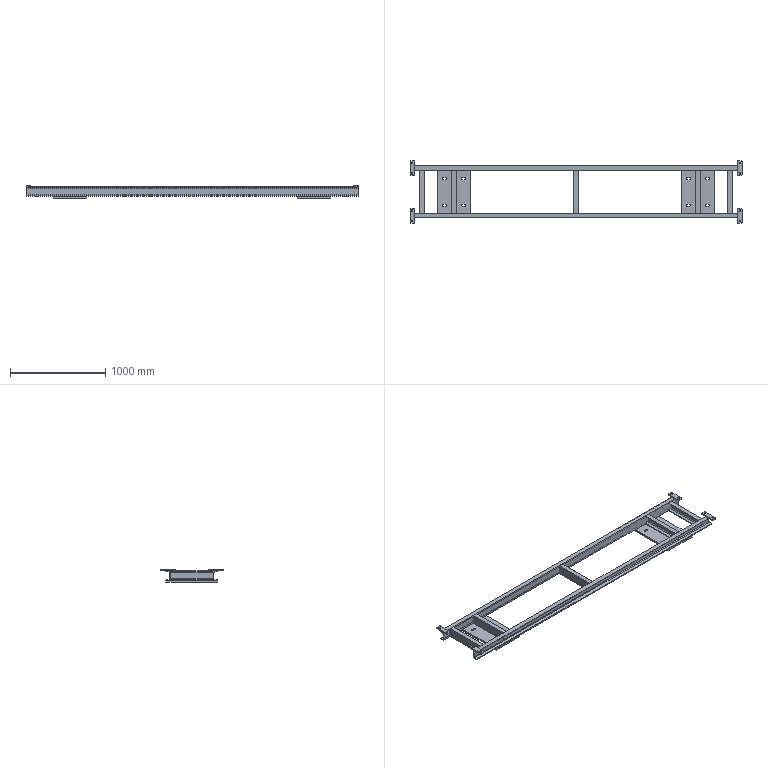Part | SolidWorks | features ICE 2, LPattern 1, MirrorPattern 1, MoveCopyBody 1, WeldMemberFeat 1, WeldmentFeature 1 | 11 solids | 222 faces | box 3487 x 660 x 134 mm | volume 19666004 mm3 | plane 138 | cylinder 84 | commonest cylinder face diameters 22 x24 14 x16 20 x16 8.4 x14 17 x14